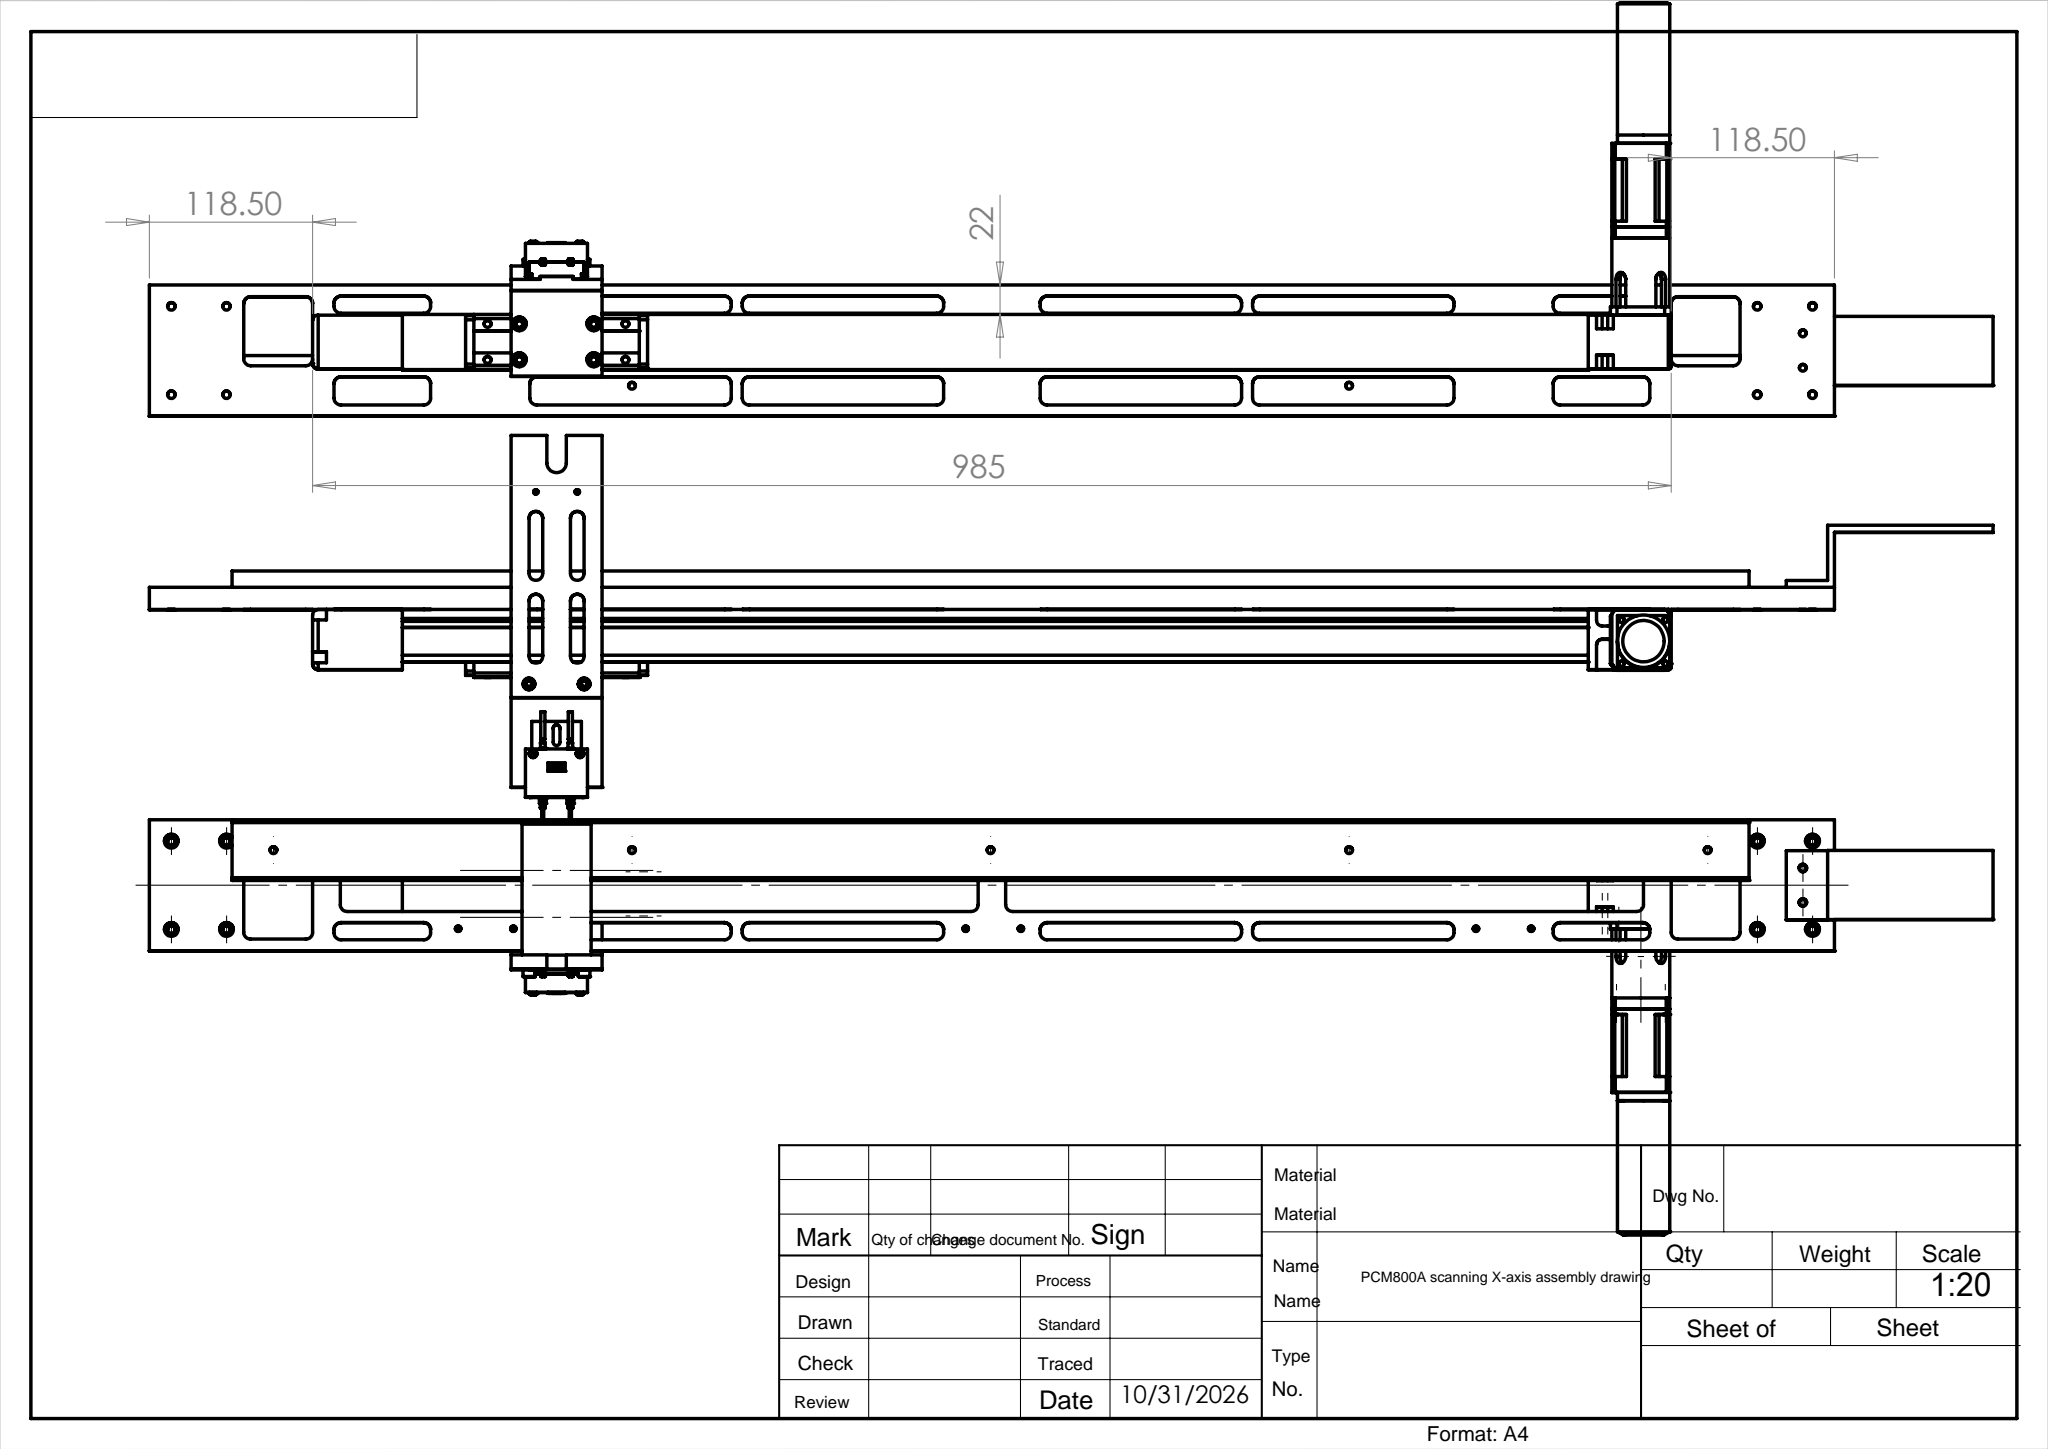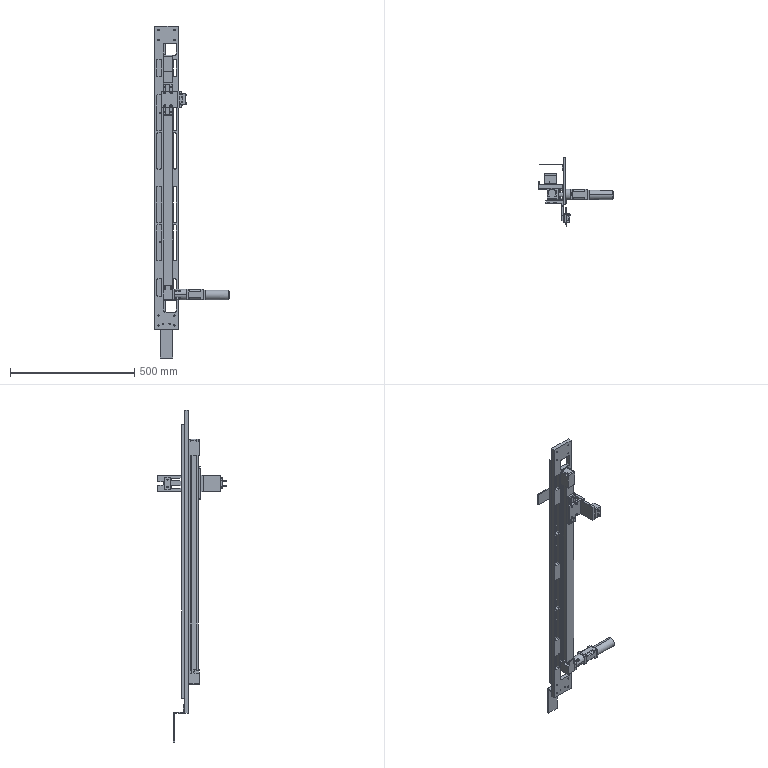Part | SolidWorks | features CompositeCurve 1 | 27 solids | 1335 faces | box 300.5 x 279.222 x 1337 mm | volume 3097922 mm3 | plane 604 | cylinder 567 | cone 96 | torus 40 | sphere 28 | commonest cylinder face diameters 10 x100 0.16 x52 5 x48 3.3 x42 4 x34 0.2 x32